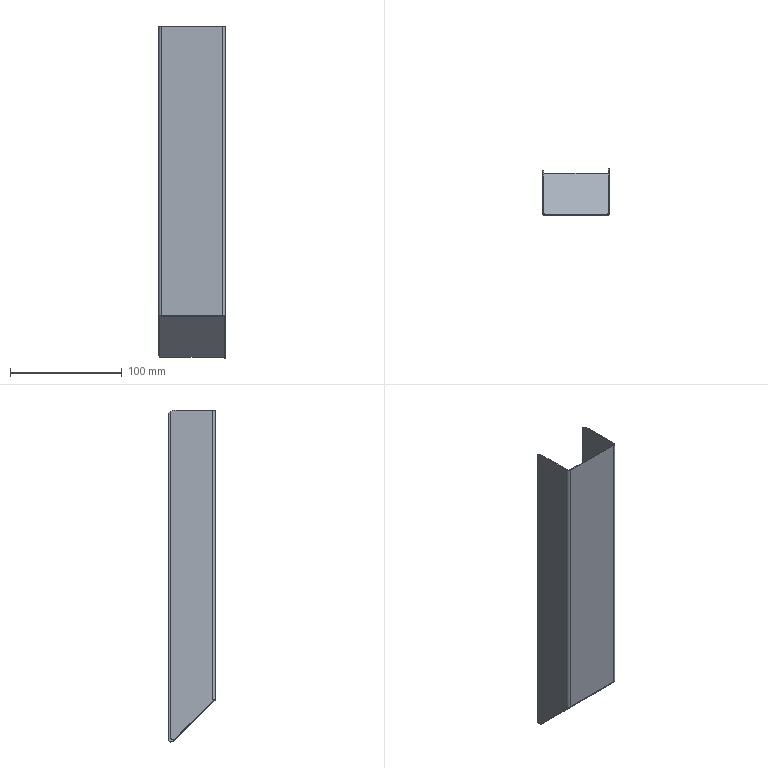Part | NX | 1 solid | 38 faces | box 60 x 42 x 297.657 mm | volume 40451 mm3 | plane 24 | cylinder 14 | commonest cylinder face diameters 4.5 x4 3.2 x2 4 x2 5.2 x2 20 x2 0.8 x1
STEP:
#1=CARTESIAN_POINT('',(1970.571,-113.09,-728.576));
#2=VERTEX_POINT('',#1);
#3=CARTESIAN_POINT('',(1970.571,-112.383,-727.869));
#4=VERTEX_POINT('',#3);
#5=CARTESIAN_POINT('',(1970.571,-112.383,-727.869));
#6=DIRECTION('',(0.,0.7071,0.7071));
#7=VECTOR('',#6,1000.);
#8=LINE('',#5,#7);
#9=EDGE_CURVE('',#2,#4,#8,.T.);
#10=ORIENTED_EDGE('',*,*,#9,.T.);
#11=CARTESIAN_POINT('',(1970.571,-75.621,-764.631));
#12=VERTEX_POINT('',#11);
#13=CARTESIAN_POINT('',(1970.571,-840.252,0.));
#14=DIRECTION('',(0.,-0.7071,0.7071));
#15=VECTOR('',#14,1000.);
#16=LINE('',#13,#15);
#17=EDGE_CURVE('',#12,#4,#16,.T.);
#18=ORIENTED_EDGE('',*,*,#17,.F.);
#19=CARTESIAN_POINT('',(1970.571,-76.328,-765.338));
#20=VERTEX_POINT('',#19);
#21=CARTESIAN_POINT('',(1970.571,0.,-689.01));
#22=DIRECTION('',(0.,-0.7071,-0.7071));
#23=VECTOR('',#22,1000.);
#24=LINE('',#21,#23);
#25=EDGE_CURVE('',#12,#20,#24,.T.);
#26=ORIENTED_EDGE('',*,*,#25,.T.);
#27=CARTESIAN_POINT('',(1970.571,-841.666,0.));
#28=DIRECTION('',(0.,-0.7071,0.7071));
#29=VECTOR('',#28,1000.);
#30=LINE('',#27,#29);
#31=EDGE_CURVE('',#20,#2,#30,.T.);
#32=ORIENTED_EDGE('',*,*,#31,.T.);
#33=EDGE_LOOP('',(#10,#18,#26,#32));
#34=FACE_BOUND('',#33,.T.);
#35=CARTESIAN_POINT('',(1970.571,-94.91,-745.342));
#36=DIRECTION('',(-1.,0.,0.));
#37=DIRECTION('',(0.,0.,1.));
#38=AXIS2_PLACEMENT_3D('',#35,#36,#37);
#39=PLANE('',#38);
#40=ADVANCED_FACE('',(#34),#39,.T.);
#41=CARTESIAN_POINT('',(2028.429,-112.383,-727.869));
#42=VERTEX_POINT('',#41);
#43=CARTESIAN_POINT('',(2028.429,-113.09,-728.576));
#44=VERTEX_POINT('',#43);
#45=CARTESIAN_POINT('',(2028.429,-112.383,-727.869));
#46=DIRECTION('',(0.,-0.7071,-0.7071));
#47=VECTOR('',#46,1000.);
#48=LINE('',#45,#47);
#49=EDGE_CURVE('',#42,#44,#48,.T.);
#50=ORIENTED_EDGE('',*,*,#49,.T.);
#51=CARTESIAN_POINT('',(2028.429,-76.328,-765.338));
#52=VERTEX_POINT('',#51);
#53=CARTESIAN_POINT('',(2028.429,-841.666,0.));
#54=DIRECTION('',(0.,0.7071,-0.7071));
#55=VECTOR('',#54,1000.);
#56=LINE('',#53,#55);
#57=EDGE_CURVE('',#44,#52,#56,.T.);
#58=ORIENTED_EDGE('',*,*,#57,.T.);
#59=CARTESIAN_POINT('',(2028.429,-75.621,-764.631));
#60=VERTEX_POINT('',#59);
#61=CARTESIAN_POINT('',(2028.429,0.,-689.01));
#62=DIRECTION('',(0.,0.7071,0.7071));
#63=VECTOR('',#62,1000.);
#64=LINE('',#61,#63);
#65=EDGE_CURVE('',#52,#60,#64,.T.);
#66=ORIENTED_EDGE('',*,*,#65,.T.);
#67=CARTESIAN_POINT('',(2028.429,-840.252,0.));
#68=DIRECTION('',(0.,0.7071,-0.7071));
#69=VECTOR('',#68,1000.);
#70=LINE('',#67,#69);
#71=EDGE_CURVE('',#42,#60,#70,.T.);
#72=ORIENTED_EDGE('',*,*,#71,.F.);
#73=EDGE_LOOP('',(#50,#58,#66,#72));
#74=FACE_BOUND('',#73,.T.);
#75=CARTESIAN_POINT('',(2028.429,-94.91,-745.342));
#76=DIRECTION('',(1.,0.,0.));
#77=DIRECTION('',(0.,1.,0.));
#78=AXIS2_PLACEMENT_3D('',#75,#76,#77);
#79=PLANE('',#78);
#80=ADVANCED_FACE('',(#74),#79,.T.);
#81=CARTESIAN_POINT('',(2026.9,-113.09,-728.576));
#82=VERTEX_POINT('',#81);
#83=CARTESIAN_POINT('',(2026.9,-113.5,-727.586));
#84=VERTEX_POINT('',#83);
#85=CARTESIAN_POINT('',(2026.9,-112.1,-727.586));
#86=DIRECTION('',(-1.,0.,0.));
#87=DIRECTION('',(0.,-0.7071,-0.7071));
#88=AXIS2_PLACEMENT_3D('',#85,#86,#87);
#89=CIRCLE('',#88,1.4);
#90=EDGE_CURVE('',#82,#84,#89,.T.);
#91=ORIENTED_EDGE('',*,*,#90,.F.);
#92=CARTESIAN_POINT('',(2026.9,-112.383,-727.869));
#93=VERTEX_POINT('',#92);
#94=CARTESIAN_POINT('',(2026.9,-113.09,-728.576));
#95=DIRECTION('',(0.,0.7071,0.7071));
#96=VECTOR('',#95,1000.);
#97=LINE('',#94,#96);
#98=EDGE_CURVE('',#82,#93,#97,.T.);
#99=ORIENTED_EDGE('',*,*,#98,.T.);
#100=CARTESIAN_POINT('',(2026.9,-112.5,-727.586));
#101=VERTEX_POINT('',#100);
#102=CARTESIAN_POINT('',(2026.9,-112.1,-727.586));
#103=DIRECTION('',(1.,0.,0.));
#104=DIRECTION('',(0.,-1.,0.));
#105=AXIS2_PLACEMENT_3D('',#102,#103,#104);
#106=CIRCLE('',#105,0.4);
#107=EDGE_CURVE('',#101,#93,#106,.T.);
#108=ORIENTED_EDGE('',*,*,#107,.F.);
#109=CARTESIAN_POINT('',(2026.9,-113.5,-727.586));
#110=DIRECTION('',(0.,1.,0.));
#111=VECTOR('',#110,1000.);
#112=LINE('',#109,#111);
#113=EDGE_CURVE('',#84,#101,#112,.T.);
#114=ORIENTED_EDGE('',*,*,#113,.F.);
#115=EDGE_LOOP('',(#91,#99,#108,#114));
#116=FACE_BOUND('',#115,.T.);
#117=CARTESIAN_POINT('',(2026.9,-112.1,-727.586));
#118=DIRECTION('',(-1.,0.,0.));
#119=DIRECTION('',(0.,0.,1.));
#120=AXIS2_PLACEMENT_3D('',#117,#118,#119);
#121=PLANE('',#120);
#122=ADVANCED_FACE('',(#116),#121,.F.);
#123=ORIENTED_EDGE('',*,*,#90,.T.);
#124=CARTESIAN_POINT('',(1972.1,-113.5,-727.586));
#125=VERTEX_POINT('',#124);
#126=CARTESIAN_POINT('',(1649.5,-113.5,-727.586));
#127=DIRECTION('',(1.,0.,0.));
#128=VECTOR('',#127,1000.);
#129=LINE('',#126,#128);
#130=EDGE_CURVE('',#125,#84,#129,.T.);
#131=ORIENTED_EDGE('',*,*,#130,.F.);
#132=CARTESIAN_POINT('',(1972.1,-113.09,-728.576));
#133=VERTEX_POINT('',#132);
#134=CARTESIAN_POINT('',(1972.1,-112.1,-727.586));
#135=DIRECTION('',(1.,0.,0.));
#136=DIRECTION('',(0.,-1.,0.));
#137=AXIS2_PLACEMENT_3D('',#134,#135,#136);
#138=CIRCLE('',#137,1.4);
#139=EDGE_CURVE('',#125,#133,#138,.T.);
#140=ORIENTED_EDGE('',*,*,#139,.T.);
#141=CARTESIAN_POINT('',(1649.5,-113.09,-728.576));
#142=DIRECTION('',(1.,0.,0.));
#143=VECTOR('',#142,1000.);
#144=LINE('',#141,#143);
#145=EDGE_CURVE('',#133,#82,#144,.T.);
#146=ORIENTED_EDGE('',*,*,#145,.T.);
#147=EDGE_LOOP('',(#123,#131,#140,#146));
#148=FACE_BOUND('',#147,.T.);
#149=CARTESIAN_POINT('',(1972.1,-112.1,-727.586));
#150=DIRECTION('',(-1.,0.,0.));
#151=DIRECTION('',(0.,0.,-1.));
#152=AXIS2_PLACEMENT_3D('',#149,#150,#151);
#153=CYLINDRICAL_SURFACE('',#152,1.4);
#154=ADVANCED_FACE('',(#148),#153,.T.);
#155=CARTESIAN_POINT('',(1649.5,-113.09,-728.576));
#156=DIRECTION('',(-1.,0.,0.));
#157=VECTOR('',#156,1000.);
#158=LINE('',#155,#157);
#159=EDGE_CURVE('',#44,#82,#158,.T.);
#160=ORIENTED_EDGE('',*,*,#159,.T.);
#161=ORIENTED_EDGE('',*,*,#145,.F.);
#162=CARTESIAN_POINT('',(1649.5,-113.09,-728.576));
#163=DIRECTION('',(-1.,0.,0.));
#164=VECTOR('',#163,1000.);
#165=LINE('',#162,#164);
#166=EDGE_CURVE('',#133,#2,#165,.T.);
#167=ORIENTED_EDGE('',*,*,#166,.T.);
#168=ORIENTED_EDGE('',*,*,#31,.F.);
#169=CARTESIAN_POINT('',(0.,-76.328,-765.338));
#170=DIRECTION('',(-1.,0.,0.));
#171=VECTOR('',#170,1000.);
#172=LINE('',#169,#171);
#173=EDGE_CURVE('',#52,#20,#172,.T.);
#174=ORIENTED_EDGE('',*,*,#173,.F.);
#175=ORIENTED_EDGE('',*,*,#57,.F.);
#176=EDGE_LOOP('',(#160,#161,#167,#168,#174,#175));
#177=FACE_BOUND('',#176,.T.);
#178=CARTESIAN_POINT('',(1649.5,-325.159,-516.507));
#179=DIRECTION('',(0.,0.7071,0.7071));
#180=DIRECTION('',(1.,0.,0.));
#181=AXIS2_PLACEMENT_3D('',#178,#179,#180);
#182=PLANE('',#181);
#183=ADVANCED_FACE('',(#177),#182,.F.);
#184=ORIENTED_EDGE('',*,*,#166,.F.);
#185=CARTESIAN_POINT('',(1972.1,-112.383,-727.869));
#186=VERTEX_POINT('',#185);
#187=CARTESIAN_POINT('',(1972.1,-113.09,-728.576));
#188=DIRECTION('',(0.,0.7071,0.7071));
#189=VECTOR('',#188,1000.);
#190=LINE('',#187,#189);
#191=EDGE_CURVE('',#133,#186,#190,.T.);
#192=ORIENTED_EDGE('',*,*,#191,.T.);
#193=CARTESIAN_POINT('',(1649.5,-112.383,-727.869));
#194=DIRECTION('',(1.,0.,0.));
#195=VECTOR('',#194,1000.);
#196=LINE('',#193,#195);
#197=EDGE_CURVE('',#4,#186,#196,.T.);
#198=ORIENTED_EDGE('',*,*,#197,.F.);
#199=ORIENTED_EDGE('',*,*,#9,.F.);
#200=EDGE_LOOP('',(#184,#192,#198,#199));
#201=FACE_BOUND('',#200,.T.);
#202=CARTESIAN_POINT('',(1972.1,-113.09,-728.576));
#203=DIRECTION('',(0.,-0.7071,0.7071));
#204=DIRECTION('',(-1.,0.,0.));
#205=AXIS2_PLACEMENT_3D('',#202,#203,#204);
#206=PLANE('',#205);
#207=ADVANCED_FACE('',(#201),#206,.T.);
#208=ORIENTED_EDGE('',*,*,#139,.F.);
#209=CARTESIAN_POINT('',(1972.1,-112.5,-727.586));
#210=VERTEX_POINT('',#209);
#211=CARTESIAN_POINT('',(1972.1,-113.5,-727.586));
#212=DIRECTION('',(0.,1.,0.));
#213=VECTOR('',#212,1000.);
#214=LINE('',#211,#213);
#215=EDGE_CURVE('',#125,#210,#214,.T.);
#216=ORIENTED_EDGE('',*,*,#215,.T.);
#217=CARTESIAN_POINT('',(1972.1,-112.1,-727.586));
#218=DIRECTION('',(-1.,0.,0.));
#219=DIRECTION('',(0.,-0.7071,-0.7071));
#220=AXIS2_PLACEMENT_3D('',#217,#218,#219);
#221=CIRCLE('',#220,0.4);
#222=EDGE_CURVE('',#186,#210,#221,.T.);
#223=ORIENTED_EDGE('',*,*,#222,.F.);
#224=ORIENTED_EDGE('',*,*,#191,.F.);
#225=EDGE_LOOP('',(#208,#216,#223,#224));
#226=FACE_BOUND('',#225,.T.);
#227=CARTESIAN_POINT('',(1972.1,-112.1,-727.586));
#228=DIRECTION('',(1.,0.,0.));
#229=DIRECTION('',(0.,1.,0.));
#230=AXIS2_PLACEMENT_3D('',#227,#228,#229);
#231=PLANE('',#230);
#232=ADVANCED_FACE('',(#226),#231,.F.);
#233=CARTESIAN_POINT('',(1969.5,-110.9,-727.586));
#234=VERTEX_POINT('',#233);
#235=CARTESIAN_POINT('',(1972.1,-110.9,-727.586));
#236=DIRECTION('',(0.,0.,1.));
#237=DIRECTION('',(-1.,0.,0.));
#238=AXIS2_PLACEMENT_3D('',#235,#236,#237);
#239=CIRCLE('',#238,2.6);
#240=EDGE_CURVE('',#234,#125,#239,.T.);
#241=ORIENTED_EDGE('',*,*,#240,.F.);
#242=CARTESIAN_POINT('',(1970.5,-110.9,-727.586));
#243=VERTEX_POINT('',#242);
#244=CARTESIAN_POINT('',(1969.5,-110.9,-727.586));
#245=DIRECTION('',(1.,0.,0.));
#246=VECTOR('',#245,1000.);
#247=LINE('',#244,#246);
#248=EDGE_CURVE('',#234,#243,#247,.T.);
#249=ORIENTED_EDGE('',*,*,#248,.T.);
#250=CARTESIAN_POINT('',(1972.1,-110.9,-727.586));
#251=DIRECTION('',(0.,0.,-1.));
#252=DIRECTION('',(0.,-1.,0.));
#253=AXIS2_PLACEMENT_3D('',#250,#251,#252);
#254=CIRCLE('',#253,1.6);
#255=EDGE_CURVE('',#210,#243,#254,.T.);
#256=ORIENTED_EDGE('',*,*,#255,.F.);
#257=ORIENTED_EDGE('',*,*,#215,.F.);
#258=EDGE_LOOP('',(#241,#249,#256,#257));
#259=FACE_BOUND('',#258,.T.);
#260=CARTESIAN_POINT('',(1972.1,-110.9,-727.586));
#261=DIRECTION('',(0.,0.,1.));
#262=DIRECTION('',(1.,0.,0.));
#263=AXIS2_PLACEMENT_3D('',#260,#261,#262);
#264=PLANE('',#263);
#265=ADVANCED_FACE('',(#259),#264,.F.);
#266=CARTESIAN_POINT('',(1972.1,-113.5,-468.166));
#267=VERTEX_POINT('',#266);
#268=CARTESIAN_POINT('',(1972.1,-113.5,-428.166));
#269=DIRECTION('',(0.,0.,-1.));
#270=VECTOR('',#269,1000.);
#271=LINE('',#268,#270);
#272=EDGE_CURVE('',#267,#125,#271,.T.);
#273=ORIENTED_EDGE('',*,*,#272,.F.);
#274=CARTESIAN_POINT('',(1969.5,-110.9,-468.166));
#275=VERTEX_POINT('',#274);
#276=CARTESIAN_POINT('',(1972.1,-110.9,-468.166));
#277=DIRECTION('',(0.,0.,1.));
#278=DIRECTION('',(-1.,0.,0.));
#279=AXIS2_PLACEMENT_3D('',#276,#277,#278);
#280=CIRCLE('',#279,2.6);
#281=EDGE_CURVE('',#275,#267,#280,.T.);
#282=ORIENTED_EDGE('',*,*,#281,.F.);
#283=CARTESIAN_POINT('',(1969.5,-110.9,-578.166));
#284=DIRECTION('',(0.,0.,1.));
#285=VECTOR('',#284,1000.);
#286=LINE('',#283,#285);
#287=EDGE_CURVE('',#234,#275,#286,.T.);
#288=ORIENTED_EDGE('',*,*,#287,.F.);
#289=ORIENTED_EDGE('',*,*,#240,.T.);
#290=EDGE_LOOP('',(#273,#282,#288,#289));
#291=FACE_BOUND('',#290,.T.);
#292=CARTESIAN_POINT('',(1972.1,-110.9,-578.166));
#293=DIRECTION('',(0.,0.,1.));
#294=DIRECTION('',(-1.,0.,0.));
#295=AXIS2_PLACEMENT_3D('',#292,#293,#294);
#296=CYLINDRICAL_SURFACE('',#295,2.6);
#297=ADVANCED_FACE('',(#291),#296,.T.);
#298=ORIENTED_EDGE('',*,*,#287,.T.);
#299=CARTESIAN_POINT('',(1969.5,-78.5,-468.166));
#300=VERTEX_POINT('',#299);
#301=CARTESIAN_POINT('',(1969.5,-112.5,-468.166));
#302=DIRECTION('',(0.,-1.,0.));
#303=VECTOR('',#302,1000.);
#304=LINE('',#301,#303);
#305=EDGE_CURVE('',#300,#275,#304,.T.);
#306=ORIENTED_EDGE('',*,*,#305,.F.);
#307=CARTESIAN_POINT('',(1969.5,-73.5,-469.506));
#308=VERTEX_POINT('',#307);
#309=CARTESIAN_POINT('',(1969.5,-78.5,-478.166));
#310=DIRECTION('',(1.,0.,0.));
#311=DIRECTION('',(0.,0.,1.));
#312=AXIS2_PLACEMENT_3D('',#309,#310,#311);
#313=CIRCLE('',#312,10.);
#314=EDGE_CURVE('',#308,#300,#313,.T.);
#315=ORIENTED_EDGE('',*,*,#314,.F.);
#316=CARTESIAN_POINT('',(1969.5,-73.5,-761.824));
#317=VERTEX_POINT('',#316);
#318=CARTESIAN_POINT('',(1969.5,-73.5,0.));
#319=DIRECTION('',(0.,0.,1.));
#320=VECTOR('',#319,1000.);
#321=LINE('',#318,#320);
#322=EDGE_CURVE('',#317,#308,#321,.T.);
#323=ORIENTED_EDGE('',*,*,#322,.F.);
#324=CARTESIAN_POINT('',(1969.5,-76.914,-763.238));
#325=VERTEX_POINT('',#324);
#326=CARTESIAN_POINT('',(1969.5,-75.5,-761.824));
#327=DIRECTION('',(1.,0.,0.));
#328=DIRECTION('',(0.,-1.,0.));
#329=AXIS2_PLACEMENT_3D('',#326,#327,#328);
#330=CIRCLE('',#329,2.);
#331=EDGE_CURVE('',#325,#317,#330,.T.);
#332=ORIENTED_EDGE('',*,*,#331,.F.);
#333=CARTESIAN_POINT('',(1969.5,-110.9,-729.252));
#334=VERTEX_POINT('',#333);
#335=CARTESIAN_POINT('',(1969.5,0.,-840.152));
#336=DIRECTION('',(0.,0.7071,-0.7071));
#337=VECTOR('',#336,1000.);
#338=LINE('',#335,#337);
#339=EDGE_CURVE('',#334,#325,#338,.T.);
#340=ORIENTED_EDGE('',*,*,#339,.F.);
#341=CARTESIAN_POINT('',(1969.5,-110.9,-428.166));
#342=DIRECTION('',(0.,0.,-1.));
#343=VECTOR('',#342,1000.);
#344=LINE('',#341,#343);
#345=EDGE_CURVE('',#234,#334,#344,.T.);
#346=ORIENTED_EDGE('',*,*,#345,.F.);
#347=EDGE_LOOP('',(#298,#306,#315,#323,#332,#340,#346));
#348=FACE_BOUND('',#347,.T.);
#349=CARTESIAN_POINT('',(1969.5,208.6,-428.166));
#350=DIRECTION('',(1.,0.,0.));
#351=DIRECTION('',(0.,1.,0.));
#352=AXIS2_PLACEMENT_3D('',#349,#350,#351);
#353=PLANE('',#352);
#354=ADVANCED_FACE('',(#348),#353,.F.);
#355=ORIENTED_EDGE('',*,*,#173,.T.);
#356=ORIENTED_EDGE('',*,*,#25,.F.);
#357=CARTESIAN_POINT('',(0.,-75.621,-764.631));
#358=DIRECTION('',(-1.,0.,0.));
#359=VECTOR('',#358,1000.);
#360=LINE('',#357,#359);
#361=EDGE_CURVE('',#60,#12,#360,.T.);
#362=ORIENTED_EDGE('',*,*,#361,.F.);
#363=ORIENTED_EDGE('',*,*,#65,.F.);
#364=EDGE_LOOP('',(#355,#356,#362,#363));
#365=FACE_BOUND('',#364,.T.);
#366=CARTESIAN_POINT('',(1969.5,-76.328,-765.338));
#367=DIRECTION('',(0.,0.7071,-0.7071));
#368=DIRECTION('',(-1.,0.,0.));
#369=AXIS2_PLACEMENT_3D('',#366,#367,#368);
#370=PLANE('',#369);
#371=ADVANCED_FACE('',(#365),#370,.T.);
#372=CARTESIAN_POINT('',(1970.5,-76.914,-763.238));
#373=VERTEX_POINT('',#372);
#374=CARTESIAN_POINT('',(0.,-76.914,-763.238));
#375=DIRECTION('',(1.,0.,0.));
#376=VECTOR('',#375,1000.);
#377=LINE('',#374,#376);
#378=EDGE_CURVE('',#325,#373,#377,.T.);
#379=ORIENTED_EDGE('',*,*,#378,.T.);
#380=CARTESIAN_POINT('',(1970.5,-110.9,-729.252));
#381=VERTEX_POINT('',#380);
#382=CARTESIAN_POINT('',(1970.5,0.,-840.152));
#383=DIRECTION('',(0.,0.7071,-0.7071));
#384=VECTOR('',#383,1000.);
#385=LINE('',#382,#384);
#386=EDGE_CURVE('',#381,#373,#385,.T.);
#387=ORIENTED_EDGE('',*,*,#386,.F.);
#388=CARTESIAN_POINT('',(1969.5,-110.9,-729.252));
#389=DIRECTION('',(1.,0.,0.));
#390=VECTOR('',#389,1000.);
#391=LINE('',#388,#390);
#392=EDGE_CURVE('',#334,#381,#391,.T.);
#393=ORIENTED_EDGE('',*,*,#392,.F.);
#394=ORIENTED_EDGE('',*,*,#339,.T.);
#395=EDGE_LOOP('',(#379,#387,#393,#394));
#396=FACE_BOUND('',#395,.T.);
#397=CARTESIAN_POINT('',(1969.5,-68.5,-771.652));
#398=DIRECTION('',(0.,-0.7071,-0.7071));
#399=DIRECTION('',(0.,-0.7071,0.7071));
#400=AXIS2_PLACEMENT_3D('',#397,#398,#399);
#401=PLANE('',#400);
#402=ADVANCED_FACE('',(#396),#401,.T.);
#403=CARTESIAN_POINT('',(1970.5,-73.5,-469.506));
#404=VERTEX_POINT('',#403);
#405=CARTESIAN_POINT('',(1649.5,-73.5,-469.506));
#406=DIRECTION('',(1.,0.,0.));
#407=VECTOR('',#406,1000.);
#408=LINE('',#405,#407);
#409=EDGE_CURVE('',#308,#404,#408,.T.);
#410=ORIENTED_EDGE('',*,*,#409,.T.);
#411=CARTESIAN_POINT('',(1970.5,-73.5,-761.824));
#412=VERTEX_POINT('',#411);
#413=CARTESIAN_POINT('',(1970.5,-73.5,0.));
#414=DIRECTION('',(0.,0.,1.));
#415=VECTOR('',#414,1000.);
#416=LINE('',#413,#415);
#417=EDGE_CURVE('',#412,#404,#416,.T.);
#418=ORIENTED_EDGE('',*,*,#417,.F.);
#419=CARTESIAN_POINT('',(0.,-73.5,-761.824));
#420=DIRECTION('',(1.,0.,0.));
#421=VECTOR('',#420,1000.);
#422=LINE('',#419,#421);
#423=EDGE_CURVE('',#317,#412,#422,.T.);
#424=ORIENTED_EDGE('',*,*,#423,.F.);
#425=ORIENTED_EDGE('',*,*,#322,.T.);
#426=EDGE_LOOP('',(#410,#418,#424,#425));
#427=FACE_BOUND('',#426,.T.);
#428=CARTESIAN_POINT('',(1969.5,-73.5,-578.166));
#429=DIRECTION('',(0.,1.,0.));
#430=DIRECTION('',(1.,0.,0.));
#431=AXIS2_PLACEMENT_3D('',#428,#429,#430);
#432=PLANE('',#431);
#433=ADVANCED_FACE('',(#427),#432,.T.);
#434=ORIENTED_EDGE('',*,*,#345,.T.);
#435=ORIENTED_EDGE('',*,*,#392,.T.);
#436=CARTESIAN_POINT('',(1970.5,-110.9,-428.166));
#437=DIRECTION('',(0.,0.,-1.));
#438=VECTOR('',#437,1000.);
#439=LINE('',#436,#438);
#440=EDGE_CURVE('',#243,#381,#439,.T.);
#441=ORIENTED_EDGE('',*,*,#440,.F.);
#442=ORIENTED_EDGE('',*,*,#248,.F.);
#443=EDGE_LOOP('',(#434,#435,#441,#442));
#444=FACE_BOUND('',#443,.T.);
#445=CARTESIAN_POINT('',(1969.5,-110.9,-728.078));
#446=DIRECTION('',(0.,-1.,0.));
#447=DIRECTION('',(-1.,0.,0.));
#448=AXIS2_PLACEMENT_3D('',#445,#446,#447);
#449=PLANE('',#448);
#450=ADVANCED_FACE('',(#444),#449,.T.);
#451=ORIENTED_EDGE('',*,*,#409,.F.);
#452=ORIENTED_EDGE('',*,*,#314,.T.);
#453=CARTESIAN_POINT('',(1970.5,-78.5,-468.166));
#454=VERTEX_POINT('',#453);
#455=CARTESIAN_POINT('',(1649.5,-78.5,-468.166));
#456=DIRECTION('',(1.,0.,0.));
#457=VECTOR('',#456,1000.);
#458=LINE('',#455,#457);
#459=EDGE_CURVE('',#300,#454,#458,.T.);
#460=ORIENTED_EDGE('',*,*,#459,.T.);
#461=CARTESIAN_POINT('',(1970.5,-78.5,-478.166));
#462=DIRECTION('',(1.,0.,0.));
#463=DIRECTION('',(0.,0.,1.));
#464=AXIS2_PLACEMENT_3D('',#461,#462,#463);
#465=CIRCLE('',#464,10.);
#466=EDGE_CURVE('',#404,#454,#465,.T.);
#467=ORIENTED_EDGE('',*,*,#466,.F.);
#468=EDGE_LOOP('',(#451,#452,#460,#467));
#469=FACE_BOUND('',#468,.T.);
#470=CARTESIAN_POINT('',(1649.5,-78.5,-478.166));
#471=DIRECTION('',(1.,0.,0.));
#472=DIRECTION('',(0.,0.,1.));
#473=AXIS2_PLACEMENT_3D('',#470,#471,#472);
#474=CYLINDRICAL_SURFACE('',#473,10.);
#475=ADVANCED_FACE('',(#469),#474,.T.);
#476=ORIENTED_EDGE('',*,*,#159,.F.);
#477=ORIENTED_EDGE('',*,*,#49,.F.);
#478=CARTESIAN_POINT('',(1649.5,-112.383,-727.869));
#479=DIRECTION('',(1.,0.,0.));
#480=VECTOR('',#479,1000.);
#481=LINE('',#478,#480);
#482=EDGE_CURVE('',#93,#42,#481,.T.);
#483=ORIENTED_EDGE('',*,*,#482,.F.);
#484=ORIENTED_EDGE('',*,*,#98,.F.);
#485=EDGE_LOOP('',(#476,#477,#483,#484));
#486=FACE_BOUND('',#485,.T.);
#487=CARTESIAN_POINT('',(2030.,-113.09,-728.576));
#488=DIRECTION('',(0.,-0.7071,0.7071));
#489=DIRECTION('',(-1.,0.,0.));
#490=AXIS2_PLACEMENT_3D('',#487,#488,#489);
#491=PLANE('',#490);
#492=ADVANCED_FACE('',(#486),#491,.T.);
#493=CARTESIAN_POINT('',(2029.5,-110.9,-727.586));
#494=VERTEX_POINT('',#493);
#495=CARTESIAN_POINT('',(2026.9,-110.9,-727.586));
#496=DIRECTION('',(0.,0.,1.));
#497=DIRECTION('',(0.,-1.,0.));
#498=AXIS2_PLACEMENT_3D('',#495,#496,#497);
#499=CIRCLE('',#498,2.6);
#500=EDGE_CURVE('',#84,#494,#499,.T.);
#501=ORIENTED_EDGE('',*,*,#500,.F.);
#502=ORIENTED_EDGE('',*,*,#113,.T.);
#503=CARTESIAN_POINT('',(2028.5,-110.9,-727.586));
#504=VERTEX_POINT('',#503);
#505=CARTESIAN_POINT('',(2026.9,-110.9,-727.586));
#506=DIRECTION('',(0.,0.,-1.));
#507=DIRECTION('',(1.,0.,0.));
#508=AXIS2_PLACEMENT_3D('',#505,#506,#507);
#509=CIRCLE('',#508,1.6);
#510=EDGE_CURVE('',#504,#101,#509,.T.);
#511=ORIENTED_EDGE('',*,*,#510,.F.);
#512=CARTESIAN_POINT('',(2029.5,-110.9,-727.586));
#513=DIRECTION('',(-1.,0.,0.));
#514=VECTOR('',#513,1000.);
#515=LINE('',#512,#514);
#516=EDGE_CURVE('',#494,#504,#515,.T.);
#517=ORIENTED_EDGE('',*,*,#516,.F.);
#518=EDGE_LOOP('',(#501,#502,#511,#517));
#519=FACE_BOUND('',#518,.T.);
#520=CARTESIAN_POINT('',(2026.9,-110.9,-727.586));
#521=DIRECTION('',(0.,0.,1.));
#522=DIRECTION('',(1.,0.,0.));
#523=AXIS2_PLACEMENT_3D('',#520,#521,#522);
#524=PLANE('',#523);
#525=ADVANCED_FACE('',(#519),#524,.F.);
#526=CARTESIAN_POINT('',(2028.5,-74.914,-765.238));
#527=VERTEX_POINT('',#526);
#528=CARTESIAN_POINT('',(2029.5,-74.914,-765.238));
#529=VERTEX_POINT('',#528);
#530=CARTESIAN_POINT('',(0.,-74.914,-765.238));
#531=DIRECTION('',(1.,0.,0.));
#532=VECTOR('',#531,1000.);
#533=LINE('',#530,#532);
#534=EDGE_CURVE('',#527,#529,#533,.T.);
#535=ORIENTED_EDGE('',*,*,#534,.T.);
#536=CARTESIAN_POINT('',(2029.5,-110.9,-729.252));
#537=VERTEX_POINT('',#536);
#538=CARTESIAN_POINT('',(2029.5,-840.152,0.));
#539=DIRECTION('',(0.,-0.7071,0.7071));
#540=VECTOR('',#539,1000.);
#541=LINE('',#538,#540);
#542=EDGE_CURVE('',#529,#537,#541,.T.);
#543=ORIENTED_EDGE('',*,*,#542,.T.);
#544=CARTESIAN_POINT('',(2028.5,-110.9,-729.252));
#545=VERTEX_POINT('',#544);
#546=CARTESIAN_POINT('',(2029.5,-110.9,-729.252));
#547=DIRECTION('',(1.,0.,0.));
#548=VECTOR('',#547,1000.);
#549=LINE('',#546,#548);
#550=EDGE_CURVE('',#545,#537,#549,.T.);
#551=ORIENTED_EDGE('',*,*,#550,.F.);
#552=CARTESIAN_POINT('',(2028.5,-840.152,0.));
#553=DIRECTION('',(0.,-0.7071,0.7071));
#554=VECTOR('',#553,1000.);
#555=LINE('',#552,#554);
#556=EDGE_CURVE('',#527,#545,#555,.T.);
#557=ORIENTED_EDGE('',*,*,#556,.F.);
#558=EDGE_LOOP('',(#535,#543,#551,#557));
#559=FACE_BOUND('',#558,.T.);
#560=CARTESIAN_POINT('',(2029.5,-111.4,-728.752));
#561=DIRECTION('',(0.,-0.7071,-0.7071));
#562=DIRECTION('',(0.,0.7071,-0.7071));
#563=AXIS2_PLACEMENT_3D('',#560,#561,#562);
#564=PLANE('',#563);
#565=ADVANCED_FACE('',(#559),#564,.T.);
#566=CARTESIAN_POINT('',(2029.5,-71.5,-763.824));
#567=VERTEX_POINT('',#566);
#568=CARTESIAN_POINT('',(2029.5,-71.5,-471.025));
#569=VERTEX_POINT('',#568);
#570=CARTESIAN_POINT('',(2029.5,-71.5,0.));
#571=DIRECTION('',(0.,0.,1.));
#572=VECTOR('',#571,1000.);
#573=LINE('',#570,#572);
#574=EDGE_CURVE('',#567,#569,#573,.T.);
#575=ORIENTED_EDGE('',*,*,#574,.F.);
#576=CARTESIAN_POINT('',(2028.5,-71.5,-763.824));
#577=VERTEX_POINT('',#576);
#578=CARTESIAN_POINT('',(0.,-71.5,-763.824));
#579=DIRECTION('',(1.,0.,0.));
#580=VECTOR('',#579,1000.);
#581=LINE('',#578,#580);
#582=EDGE_CURVE('',#577,#567,#581,.T.);
#583=ORIENTED_EDGE('',*,*,#582,.F.);
#584=CARTESIAN_POINT('',(2028.5,-71.5,-471.025));
#585=VERTEX_POINT('',#584);
#586=CARTESIAN_POINT('',(2028.5,-71.5,0.));
#587=DIRECTION('',(0.,0.,-1.));
#588=VECTOR('',#587,1000.);
#589=LINE('',#586,#588);
#590=EDGE_CURVE('',#585,#577,#589,.T.);
#591=ORIENTED_EDGE('',*,*,#590,.F.);
#592=CARTESIAN_POINT('',(1649.5,-71.5,-471.025));
#593=DIRECTION('',(1.,0.,0.));
#594=VECTOR('',#593,1000.);
#595=LINE('',#592,#594);
#596=EDGE_CURVE('',#585,#569,#595,.T.);
#597=ORIENTED_EDGE('',*,*,#596,.T.);
#598=EDGE_LOOP('',(#575,#583,#591,#597));
#599=FACE_BOUND('',#598,.T.);
#600=CARTESIAN_POINT('',(2029.5,-71.5,-771.652));
#601=DIRECTION('',(0.,1.,0.));
#602=DIRECTION('',(1.,0.,0.));
#603=AXIS2_PLACEMENT_3D('',#600,#601,#602);
#604=PLANE('',#603);
#605=ADVANCED_FACE('',(#599),#604,.T.);
#606=ORIENTED_EDGE('',*,*,#500,.T.);
#607=CARTESIAN_POINT('',(2029.5,-110.9,-468.166));
#608=VERTEX_POINT('',#607);
#609=CARTESIAN_POINT('',(2029.5,-110.9,-727.586));
#610=DIRECTION('',(0.,0.,-1.));
#611=VECTOR('',#610,1000.);
#612=LINE('',#609,#611);
#613=EDGE_CURVE('',#608,#494,#612,.T.);
#614=ORIENTED_EDGE('',*,*,#613,.F.);
#615=CARTESIAN_POINT('',(2026.9,-113.5,-468.166));
#616=VERTEX_POINT('',#615);
#617=CARTESIAN_POINT('',(2026.9,-110.9,-468.166));
#618=DIRECTION('',(0.,0.,-1.));
#619=DIRECTION('',(1.,0.,0.));
#620=AXIS2_PLACEMENT_3D('',#617,#618,#619);
#621=CIRCLE('',#620,2.6);
#622=EDGE_CURVE('',#608,#616,#621,.T.);
#623=ORIENTED_EDGE('',*,*,#622,.T.);
#624=CARTESIAN_POINT('',(2026.9,-113.5,-428.166));
#625=DIRECTION('',(0.,0.,-1.));
#626=VECTOR('',#625,1000.);
#627=LINE('',#624,#626);
#628=EDGE_CURVE('',#616,#84,#627,.T.);
#629=ORIENTED_EDGE('',*,*,#628,.T.);
#630=EDGE_LOOP('',(#606,#614,#623,#629));
#631=FACE_BOUND('',#630,.T.);
#632=CARTESIAN_POINT('',(2026.9,-110.9,-727.586));
#633=DIRECTION('',(0.,0.,-1.));
#634=DIRECTION('',(1.,0.,0.));
#635=AXIS2_PLACEMENT_3D('',#632,#633,#634);
#636=CYLINDRICAL_SURFACE('',#635,2.6);
#637=ADVANCED_FACE('',(#631),#636,.T.);
#638=CARTESIAN_POINT('',(2028.5,-78.5,-468.166));
#639=VERTEX_POINT('',#638);
#640=CARTESIAN_POINT('',(2029.5,-78.5,-468.166));
#641=VERTEX_POINT('',#640);
#642=CARTESIAN_POINT('',(1649.5,-78.5,-468.166));
#643=DIRECTION('',(1.,0.,0.));
#644=VECTOR('',#643,1000.);
#645=LINE('',#642,#644);
#646=EDGE_CURVE('',#639,#641,#645,.T.);
#647=ORIENTED_EDGE('',*,*,#646,.F.);
#648=CARTESIAN_POINT('',(2028.5,-110.9,-468.166));
#649=VERTEX_POINT('',#648);
#650=CARTESIAN_POINT('',(2028.5,-112.5,-468.166));
#651=DIRECTION('',(0.,1.,0.));
#652=VECTOR('',#651,1000.);
#653=LINE('',#650,#652);
#654=EDGE_CURVE('',#649,#639,#653,.T.);
#655=ORIENTED_EDGE('',*,*,#654,.F.);
#656=CARTESIAN_POINT('',(2026.9,-112.5,-468.166));
#657=VERTEX_POINT('',#656);
#658=CARTESIAN_POINT('',(2026.9,-110.9,-468.166));
#659=DIRECTION('',(0.,0.,-1.));
#660=DIRECTION('',(1.,0.,0.));
#661=AXIS2_PLACEMENT_3D('',#658,#659,#660);
#662=CIRCLE('',#661,1.6);
#663=EDGE_CURVE('',#649,#657,#662,.T.);
#664=ORIENTED_EDGE('',*,*,#663,.T.);
#665=CARTESIAN_POINT('',(1972.1,-112.5,-468.166));
#666=VERTEX_POINT('',#665);
#667=CARTESIAN_POINT('',(1649.5,-112.5,-468.166));
#668=DIRECTION('',(1.,0.,0.));
#669=VECTOR('',#668,1000.);
#670=LINE('',#667,#669);
#671=EDGE_CURVE('',#666,#657,#670,.T.);
#672=ORIENTED_EDGE('',*,*,#671,.F.);
#673=CARTESIAN_POINT('',(1970.5,-110.9,-468.166));
#674=VERTEX_POINT('',#673);
#675=CARTESIAN_POINT('',(1972.1,-110.9,-468.166));
#676=DIRECTION('',(0.,0.,1.));
#677=DIRECTION('',(-1.,0.,0.));
#678=AXIS2_PLACEMENT_3D('',#675,#676,#677);
#679=CIRCLE('',#678,1.6);
#680=EDGE_CURVE('',#674,#666,#679,.T.);
#681=ORIENTED_EDGE('',*,*,#680,.F.);
#682=CARTESIAN_POINT('',(1970.5,-112.5,-468.166));
#683=DIRECTION('',(0.,-1.,0.));
#684=VECTOR('',#683,1000.);
#685=LINE('',#682,#684);
#686=EDGE_CURVE('',#454,#674,#685,.T.);
#687=ORIENTED_EDGE('',*,*,#686,.F.);
#688=ORIENTED_EDGE('',*,*,#459,.F.);
#689=ORIENTED_EDGE('',*,*,#305,.T.);
#690=ORIENTED_EDGE('',*,*,#281,.T.);
#691=CARTESIAN_POINT('',(1649.5,-113.5,-468.166));
#692=DIRECTION('',(-1.,0.,0.));
#693=VECTOR('',#692,1000.);
#694=LINE('',#691,#693);
#695=EDGE_CURVE('',#616,#267,#694,.T.);
#696=ORIENTED_EDGE('',*,*,#695,.F.);
#697=ORIENTED_EDGE('',*,*,#622,.F.);
#698=CARTESIAN_POINT('',(2029.5,-112.5,-468.166));
#699=DIRECTION('',(0.,-1.,0.));
#700=VECTOR('',#699,1000.);
#701=LINE('',#698,#700);
#702=EDGE_CURVE('',#641,#608,#701,.T.);
#703=ORIENTED_EDGE('',*,*,#702,.F.);
#704=EDGE_LOOP('',(#647,#655,#664,#672,#681,#687,#688,#689,#690,#696,#697,#703));
#705=FACE_BOUND('',#704,.T.);
#706=CARTESIAN_POINT('',(2029.5,-68.5,-468.166));
#707=DIRECTION('',(0.,0.,1.));
#708=DIRECTION('',(0.,-1.,0.));
#709=AXIS2_PLACEMENT_3D('',#706,#707,#708);
#710=PLANE('',#709);
#711=ADVANCED_FACE('',(#705),#710,.T.);
#712=CARTESIAN_POINT('',(2029.5,-110.9,-428.166));
#713=DIRECTION('',(0.,0.,-1.));
#714=VECTOR('',#713,1000.);
#715=LINE('',#712,#714);
#716=EDGE_CURVE('',#494,#537,#715,.T.);
#717=ORIENTED_EDGE('',*,*,#716,.F.);
#718=ORIENTED_EDGE('',*,*,#516,.T.);
#719=CARTESIAN_POINT('',(2028.5,-110.9,-428.166));
#720=DIRECTION('',(0.,0.,1.));
#721=VECTOR('',#720,1000.);
#722=LINE('',#719,#721);
#723=EDGE_CURVE('',#545,#504,#722,.T.);
#724=ORIENTED_EDGE('',*,*,#723,.F.);
#725=ORIENTED_EDGE('',*,*,#550,.T.);
#726=EDGE_LOOP('',(#717,#718,#724,#725));
#727=FACE_BOUND('',#726,.T.);
#728=CARTESIAN_POINT('',(2029.5,-110.9,-727.586));
#729=DIRECTION('',(0.,-1.,0.));
#730=DIRECTION('',(-1.,0.,0.));
#731=AXIS2_PLACEMENT_3D('',#728,#729,#730);
#732=PLANE('',#731);
#733=ADVANCED_FACE('',(#727),#732,.T.);
#734=ORIENTED_EDGE('',*,*,#628,.F.);
#735=ORIENTED_EDGE('',*,*,#695,.T.);
#736=ORIENTED_EDGE('',*,*,#272,.T.);
#737=ORIENTED_EDGE('',*,*,#130,.T.);
#738=EDGE_LOOP('',(#734,#735,#736,#737));
#739=FACE_BOUND('',#738,.T.);
#740=CARTESIAN_POINT('',(2029.5,-113.5,-578.166));
#741=DIRECTION('',(0.,-1.,0.));
#742=DIRECTION('',(0.,0.,-1.));
#743=AXIS2_PLACEMENT_3D('',#740,#741,#742);
#744=PLANE('',#743);
#745=ADVANCED_FACE('',(#739),#744,.T.);
#746=ORIENTED_EDGE('',*,*,#613,.T.);
#747=ORIENTED_EDGE('',*,*,#716,.T.);
#748=ORIENTED_EDGE('',*,*,#542,.F.);
#749=CARTESIAN_POINT('',(2029.5,-73.5,-763.824));
#750=DIRECTION('',(1.,0.,0.));
#751=DIRECTION('',(0.,-1.,0.));
#752=AXIS2_PLACEMENT_3D('',#749,#750,#751);
#753=CIRCLE('',#752,2.);
#754=EDGE_CURVE('',#529,#567,#753,.T.);
#755=ORIENTED_EDGE('',*,*,#754,.T.);
#756=ORIENTED_EDGE('',*,*,#574,.T.);
#757=CARTESIAN_POINT('',(2029.5,-78.5,-478.166));
#758=DIRECTION('',(1.,0.,0.));
#759=DIRECTION('',(0.,0.,1.));
#760=AXIS2_PLACEMENT_3D('',#757,#758,#759);
#761=CIRCLE('',#760,10.);
#762=EDGE_CURVE('',#569,#641,#761,.T.);
#763=ORIENTED_EDGE('',*,*,#762,.T.);
#764=ORIENTED_EDGE('',*,*,#702,.T.);
#765=EDGE_LOOP('',(#746,#747,#748,#755,#756,#763,#764));
#766=FACE_BOUND('',#765,.T.);
#767=CARTESIAN_POINT('',(2029.5,-103.785,-719.977));
#768=VERTEX_POINT('',#767);
#769=CARTESIAN_POINT('',(2029.5,-108.241,-719.35));
#770=VERTEX_POINT('',#769);
#771=CARTESIAN_POINT('',(2029.5,-106.013,-719.664));
#772=DIRECTION('',(-1.,0.,0.));
#773=DIRECTION('',(0.,-0.9903,0.1392));
#774=AXIS2_PLACEMENT_3D('',#771,#772,#773);
#775=CIRCLE('',#774,2.25);
#776=EDGE_CURVE('',#768,#770,#775,.T.);
#777=ORIENTED_EDGE('',*,*,#776,.T.);
#778=CARTESIAN_POINT('',(2029.5,-106.013,-719.664));
#779=DIRECTION('',(-1.,0.,0.));
#780=DIRECTION('',(0.,-0.9903,0.1392));
#781=AXIS2_PLACEMENT_3D('',#778,#779,#780);
#782=CIRCLE('',#781,2.25);
#783=EDGE_CURVE('',#770,#768,#782,.T.);
#784=ORIENTED_EDGE('',*,*,#783,.T.);
#785=EDGE_LOOP('',(#777,#784));
#786=FACE_BOUND('',#785,.T.);
#787=CARTESIAN_POINT('',(2029.5,-80.536,-683.89));
#788=VERTEX_POINT('',#787);
#789=CARTESIAN_POINT('',(2029.5,-76.08,-684.516));
#790=VERTEX_POINT('',#789);
#791=CARTESIAN_POINT('',(2029.5,-78.308,-684.203));
#792=DIRECTION('',(-1.,0.,0.));
#793=DIRECTION('',(0.,-0.9903,0.1392));
#794=AXIS2_PLACEMENT_3D('',#791,#792,#793);
#795=CIRCLE('',#794,2.25);
#796=EDGE_CURVE('',#788,#790,#795,.T.);
#797=ORIENTED_EDGE('',*,*,#796,.T.);
#798=CARTESIAN_POINT('',(2029.5,-78.308,-684.203));
#799=DIRECTION('',(-1.,0.,0.));
#800=DIRECTION('',(0.,-0.9903,0.1392));
#801=AXIS2_PLACEMENT_3D('',#798,#799,#800);
#802=CIRCLE('',#801,2.25);
#803=EDGE_CURVE('',#790,#788,#802,.T.);
#804=ORIENTED_EDGE('',*,*,#803,.T.);
#805=EDGE_LOOP('',(#797,#804));
#806=FACE_BOUND('',#805,.T.);
#807=CARTESIAN_POINT('',(2029.5,-111.4,-578.166));
#808=DIRECTION('',(1.,0.,0.));
#809=DIRECTION('',(0.,1.,0.));
#810=AXIS2_PLACEMENT_3D('',#807,#808,#809);
#811=PLANE('',#810);
#812=ADVANCED_FACE('',(#766,#786,#806),#811,.T.);
#813=ORIENTED_EDGE('',*,*,#646,.T.);
#814=ORIENTED_EDGE('',*,*,#762,.F.);
#815=ORIENTED_EDGE('',*,*,#596,.F.);
#816=CARTESIAN_POINT('',(2028.5,-78.5,-478.166));
#817=DIRECTION('',(1.,0.,0.));
#818=DIRECTION('',(0.,0.,1.));
#819=AXIS2_PLACEMENT_3D('',#816,#817,#818);
#820=CIRCLE('',#819,10.);
#821=EDGE_CURVE('',#585,#639,#820,.T.);
#822=ORIENTED_EDGE('',*,*,#821,.T.);
#823=EDGE_LOOP('',(#813,#814,#815,#822));
#824=FACE_BOUND('',#823,.T.);
#825=CARTESIAN_POINT('',(1649.5,-78.5,-478.166));
#826=DIRECTION('',(1.,0.,0.));
#827=DIRECTION('',(0.,0.,1.));
#828=AXIS2_PLACEMENT_3D('',#825,#826,#827);
#829=CYLINDRICAL_SURFACE('',#828,10.);
#830=ADVANCED_FACE('',(#824),#829,.T.);
#831=CARTESIAN_POINT('',(2028.5,-103.785,-719.977));
#832=VERTEX_POINT('',#831);
#833=CARTESIAN_POINT('',(2028.5,-108.241,-719.35));
#834=VERTEX_POINT('',#833);
#835=CARTESIAN_POINT('',(2028.5,-106.013,-719.664));
#836=DIRECTION('',(-1.,0.,0.));
#837=DIRECTION('',(0.,-0.9903,0.1392));
#838=AXIS2_PLACEMENT_3D('',#835,#836,#837);
#839=CIRCLE('',#838,2.25);
#840=EDGE_CURVE('',#832,#834,#839,.T.);
#841=ORIENTED_EDGE('',*,*,#840,.T.);
#842=CARTESIAN_POINT('',(2035.5,-108.241,-719.35));
#843=DIRECTION('',(-1.,0.,0.));
#844=VECTOR('',#843,1000.);
#845=LINE('',#842,#844);
#846=EDGE_CURVE('',#770,#834,#845,.T.);
#847=ORIENTED_EDGE('',*,*,#846,.F.);
#848=ORIENTED_EDGE('',*,*,#776,.F.);
#849=CARTESIAN_POINT('',(2035.5,-103.785,-719.977));
#850=DIRECTION('',(-1.,0.,0.));
#851=VECTOR('',#850,1000.);
#852=LINE('',#849,#851);
#853=EDGE_CURVE('',#768,#832,#852,.T.);
#854=ORIENTED_EDGE('',*,*,#853,.T.);
#855=EDGE_LOOP('',(#841,#847,#848,#854));
#856=FACE_BOUND('',#855,.T.);
#857=CARTESIAN_POINT('',(2035.5,-106.013,-719.664));
#858=DIRECTION('',(-1.,0.,0.));
#859=DIRECTION('',(0.,-0.9903,0.1392));
#860=AXIS2_PLACEMENT_3D('',#857,#858,#859);
#861=CYLINDRICAL_SURFACE('',#860,2.25);
#862=ADVANCED_FACE('',(#856),#861,.F.);
#863=CARTESIAN_POINT('',(2028.5,-76.08,-684.516));
#864=VERTEX_POINT('',#863);
#865=CARTESIAN_POINT('',(2028.5,-80.536,-683.89));
#866=VERTEX_POINT('',#865);
#867=CARTESIAN_POINT('',(2028.5,-78.308,-684.203));
#868=DIRECTION('',(-1.,0.,0.));
#869=DIRECTION('',(0.,-0.9903,0.1392));
#870=AXIS2_PLACEMENT_3D('',#867,#868,#869);
#871=CIRCLE('',#870,2.25);
#872=EDGE_CURVE('',#864,#866,#871,.T.);
#873=ORIENTED_EDGE('',*,*,#872,.T.);
#874=CARTESIAN_POINT('',(2035.5,-80.536,-683.89));
#875=DIRECTION('',(-1.,0.,0.));
#876=VECTOR('',#875,1000.);
#877=LINE('',#874,#876);
#878=EDGE_CURVE('',#866,#788,#877,.F.);
#879=ORIENTED_EDGE('',*,*,#878,.T.);
#880=ORIENTED_EDGE('',*,*,#803,.F.);
#881=CARTESIAN_POINT('',(2035.5,-76.08,-684.516));
#882=DIRECTION('',(-1.,0.,0.));
#883=VECTOR('',#882,1000.);
#884=LINE('',#881,#883);
#885=EDGE_CURVE('',#864,#790,#884,.F.);
#886=ORIENTED_EDGE('',*,*,#885,.F.);
#887=EDGE_LOOP('',(#873,#879,#880,#886));
#888=FACE_BOUND('',#887,.T.);
#889=CARTESIAN_POINT('',(2035.5,-78.308,-684.203));
#890=DIRECTION('',(-1.,0.,0.));
#891=DIRECTION('',(0.,-0.9903,0.1392));
#892=AXIS2_PLACEMENT_3D('',#889,#890,#891);
#893=CYLINDRICAL_SURFACE('',#892,2.25);
#894=ADVANCED_FACE('',(#888),#893,.F.);
#895=ORIENTED_EDGE('',*,*,#71,.T.);
#896=ORIENTED_EDGE('',*,*,#361,.T.);
#897=ORIENTED_EDGE('',*,*,#17,.T.);
#898=ORIENTED_EDGE('',*,*,#197,.T.);
#899=CARTESIAN_POINT('',(1649.5,-112.383,-727.869));
#900=DIRECTION('',(1.,0.,0.));
#901=VECTOR('',#900,1000.);
#902=LINE('',#899,#901);
#903=EDGE_CURVE('',#186,#93,#902,.T.);
#904=ORIENTED_EDGE('',*,*,#903,.T.);
#905=ORIENTED_EDGE('',*,*,#482,.T.);
#906=EDGE_LOOP('',(#895,#896,#897,#898,#904,#905));
#907=FACE_BOUND('',#906,.T.);
#908=CARTESIAN_POINT('',(1649.5,-324.452,-515.8));
#909=DIRECTION('',(0.,0.7071,0.7071));
#910=DIRECTION('',(1.,0.,0.));
#911=AXIS2_PLACEMENT_3D('',#908,#909,#910);
#912=PLANE('',#911);
#913=ADVANCED_FACE('',(#907),#912,.T.);
#914=ORIENTED_EDGE('',*,*,#510,.T.);
#915=CARTESIAN_POINT('',(2026.9,-112.5,-428.166));
#916=DIRECTION('',(0.,0.,1.));
#917=VECTOR('',#916,1000.);
#918=LINE('',#915,#917);
#919=EDGE_CURVE('',#101,#657,#918,.T.);
#920=ORIENTED_EDGE('',*,*,#919,.T.);
#921=ORIENTED_EDGE('',*,*,#663,.F.);
#922=CARTESIAN_POINT('',(2028.5,-110.9,-727.586));
#923=DIRECTION('',(0.,0.,-1.));
#924=VECTOR('',#923,1000.);
#925=LINE('',#922,#924);
#926=EDGE_CURVE('',#649,#504,#925,.T.);
#927=ORIENTED_EDGE('',*,*,#926,.T.);
#928=EDGE_LOOP('',(#914,#920,#921,#927));
#929=FACE_BOUND('',#928,.T.);
#930=CARTESIAN_POINT('',(2026.9,-110.9,-727.586));
#931=DIRECTION('',(0.,0.,-1.));
#932=DIRECTION('',(1.,0.,0.));
#933=AXIS2_PLACEMENT_3D('',#930,#931,#932);
#934=CYLINDRICAL_SURFACE('',#933,1.6);
#935=ADVANCED_FACE('',(#929),#934,.F.);
#936=ORIENTED_EDGE('',*,*,#107,.T.);
#937=ORIENTED_EDGE('',*,*,#903,.F.);
#938=ORIENTED_EDGE('',*,*,#222,.T.);
#939=CARTESIAN_POINT('',(1649.5,-112.5,-727.586));
#940=DIRECTION('',(1.,0.,0.));
#941=VECTOR('',#940,1000.);
#942=LINE('',#939,#941);
#943=EDGE_CURVE('',#210,#101,#942,.T.);
#944=ORIENTED_EDGE('',*,*,#943,.T.);
#945=EDGE_LOOP('',(#936,#937,#938,#944));
#946=FACE_BOUND('',#945,.T.);
#947=CARTESIAN_POINT('',(1972.1,-112.1,-727.586));
#948=DIRECTION('',(-1.,0.,0.));
#949=DIRECTION('',(0.,0.,-1.));
#950=AXIS2_PLACEMENT_3D('',#947,#948,#949);
#951=CYLINDRICAL_SURFACE('',#950,0.4);
#952=ADVANCED_FACE('',(#946),#951,.F.);
#953=CARTESIAN_POINT('',(1972.1,-112.5,-428.166));
#954=DIRECTION('',(0.,0.,-1.));
#955=VECTOR('',#954,1000.);
#956=LINE('',#953,#955);
#957=EDGE_CURVE('',#666,#210,#956,.T.);
#958=ORIENTED_EDGE('',*,*,#957,.T.);
#959=ORIENTED_EDGE('',*,*,#255,.T.);
#960=CARTESIAN_POINT('',(1970.5,-110.9,-578.166));
#961=DIRECTION('',(0.,0.,1.));
#962=VECTOR('',#961,1000.);
#963=LINE('',#960,#962);
#964=EDGE_CURVE('',#243,#674,#963,.T.);
#965=ORIENTED_EDGE('',*,*,#964,.T.);
#966=ORIENTED_EDGE('',*,*,#680,.T.);
#967=EDGE_LOOP('',(#958,#959,#965,#966));
#968=FACE_BOUND('',#967,.T.);
#969=CARTESIAN_POINT('',(1972.1,-110.9,-578.166));
#970=DIRECTION('',(0.,0.,1.));
#971=DIRECTION('',(-1.,0.,0.));
#972=AXIS2_PLACEMENT_3D('',#969,#970,#971);
#973=CYLINDRICAL_SURFACE('',#972,1.6);
#974=ADVANCED_FACE('',(#968),#973,.F.);
#975=ORIENTED_EDGE('',*,*,#964,.F.);
#976=ORIENTED_EDGE('',*,*,#440,.T.);
#977=ORIENTED_EDGE('',*,*,#386,.T.);
#978=CARTESIAN_POINT('',(1970.5,-75.5,-761.824));
#979=DIRECTION('',(1.,0.,0.));
#980=DIRECTION('',(0.,-1.,0.));
#981=AXIS2_PLACEMENT_3D('',#978,#979,#980);
#982=CIRCLE('',#981,2.);
#983=EDGE_CURVE('',#373,#412,#982,.T.);
#984=ORIENTED_EDGE('',*,*,#983,.T.);
#985=ORIENTED_EDGE('',*,*,#417,.T.);
#986=ORIENTED_EDGE('',*,*,#466,.T.);
#987=ORIENTED_EDGE('',*,*,#686,.T.);
#988=EDGE_LOOP('',(#975,#976,#977,#984,#985,#986,#987));
#989=FACE_BOUND('',#988,.T.);
#990=CARTESIAN_POINT('',(1970.5,208.6,-428.166));
#991=DIRECTION('',(1.,0.,0.));
#992=DIRECTION('',(0.,1.,0.));
#993=AXIS2_PLACEMENT_3D('',#990,#991,#992);
#994=PLANE('',#993);
#995=ADVANCED_FACE('',(#989),#994,.T.);
#996=ORIENTED_EDGE('',*,*,#919,.F.);
#997=ORIENTED_EDGE('',*,*,#943,.F.);
#998=ORIENTED_EDGE('',*,*,#957,.F.);
#999=ORIENTED_EDGE('',*,*,#671,.T.);
#1000=EDGE_LOOP('',(#996,#997,#998,#999));
#1001=FACE_BOUND('',#1000,.T.);
#1002=CARTESIAN_POINT('',(1649.5,-112.5,-428.166));
#1003=DIRECTION('',(0.,1.,0.));
#1004=DIRECTION('',(1.,0.,0.));
#1005=AXIS2_PLACEMENT_3D('',#1002,#1003,#1004);
#1006=PLANE('',#1005);
#1007=ADVANCED_FACE('',(#1001),#1006,.T.);
#1008=ORIENTED_EDGE('',*,*,#926,.F.);
#1009=ORIENTED_EDGE('',*,*,#654,.T.);
#1010=ORIENTED_EDGE('',*,*,#821,.F.);
#1011=ORIENTED_EDGE('',*,*,#590,.T.);
#1012=CARTESIAN_POINT('',(2028.5,-73.5,-763.824));
#1013=DIRECTION('',(1.,0.,0.));
#1014=DIRECTION('',(0.,-1.,0.));
#1015=AXIS2_PLACEMENT_3D('',#1012,#1013,#1014);
#1016=CIRCLE('',#1015,2.);
#1017=EDGE_CURVE('',#527,#577,#1016,.T.);
#1018=ORIENTED_EDGE('',*,*,#1017,.F.);
#1019=ORIENTED_EDGE('',*,*,#556,.T.);
#1020=ORIENTED_EDGE('',*,*,#723,.T.);
#1021=EDGE_LOOP('',(#1008,#1009,#1010,#1011,#1018,#1019,#1020));
#1022=FACE_BOUND('',#1021,.T.);
#1023=ORIENTED_EDGE('',*,*,#872,.F.);
#1024=CARTESIAN_POINT('',(2028.5,-78.308,-684.203));
#1025=DIRECTION('',(-1.,0.,0.));
#1026=DIRECTION('',(0.,-0.9903,0.1392));
#1027=AXIS2_PLACEMENT_3D('',#1024,#1025,#1026);
#1028=CIRCLE('',#1027,2.25);
#1029=EDGE_CURVE('',#866,#864,#1028,.T.);
#1030=ORIENTED_EDGE('',*,*,#1029,.F.);
#1031=EDGE_LOOP('',(#1023,#1030));
#1032=FACE_BOUND('',#1031,.T.);
#1033=ORIENTED_EDGE('',*,*,#840,.F.);
#1034=CARTESIAN_POINT('',(2028.5,-106.013,-719.664));
#1035=DIRECTION('',(-1.,0.,0.));
#1036=DIRECTION('',(0.,-0.9903,0.1392));
#1037=AXIS2_PLACEMENT_3D('',#1034,#1035,#1036);
#1038=CIRCLE('',#1037,2.25);
#1039=EDGE_CURVE('',#834,#832,#1038,.T.);
#1040=ORIENTED_EDGE('',*,*,#1039,.F.);
#1041=EDGE_LOOP('',(#1033,#1040));
#1042=FACE_BOUND('',#1041,.T.);
#1043=CARTESIAN_POINT('',(2028.5,-491.4,-428.166));
#1044=DIRECTION('',(-1.,0.,0.));
#1045=DIRECTION('',(0.,0.,1.));
#1046=AXIS2_PLACEMENT_3D('',#1043,#1044,#1045);
#1047=PLANE('',#1046);
#1048=ADVANCED_FACE('',(#1022,#1032,#1042),#1047,.T.);
#1049=ORIENTED_EDGE('',*,*,#378,.F.);
#1050=ORIENTED_EDGE('',*,*,#331,.T.);
#1051=ORIENTED_EDGE('',*,*,#423,.T.);
#1052=ORIENTED_EDGE('',*,*,#983,.F.);
#1053=EDGE_LOOP('',(#1049,#1050,#1051,#1052));
#1054=FACE_BOUND('',#1053,.T.);
#1055=CARTESIAN_POINT('',(0.,-75.5,-761.824));
#1056=DIRECTION('',(1.,0.,0.));
#1057=DIRECTION('',(0.,-1.,0.));
#1058=AXIS2_PLACEMENT_3D('',#1055,#1056,#1057);
#1059=CYLINDRICAL_SURFACE('',#1058,2.);
#1060=ADVANCED_FACE('',(#1054),#1059,.T.);
#1061=ORIENTED_EDGE('',*,*,#534,.F.);
#1062=ORIENTED_EDGE('',*,*,#1017,.T.);
#1063=ORIENTED_EDGE('',*,*,#582,.T.);
#1064=ORIENTED_EDGE('',*,*,#754,.F.);
#1065=EDGE_LOOP('',(#1061,#1062,#1063,#1064));
#1066=FACE_BOUND('',#1065,.T.);
#1067=CARTESIAN_POINT('',(0.,-73.5,-763.824));
#1068=DIRECTION('',(1.,0.,0.));
#1069=DIRECTION('',(0.,-1.,0.));
#1070=AXIS2_PLACEMENT_3D('',#1067,#1068,#1069);
#1071=CYLINDRICAL_SURFACE('',#1070,2.);
#1072=ADVANCED_FACE('',(#1066),#1071,.T.);
#1073=ORIENTED_EDGE('',*,*,#796,.F.);
#1074=ORIENTED_EDGE('',*,*,#878,.F.);
#1075=ORIENTED_EDGE('',*,*,#1029,.T.);
#1076=ORIENTED_EDGE('',*,*,#885,.T.);
#1077=EDGE_LOOP('',(#1073,#1074,#1075,#1076));
#1078=FACE_BOUND('',#1077,.T.);
#1079=CARTESIAN_POINT('',(2035.5,-78.308,-684.203));
#1080=DIRECTION('',(-1.,0.,0.));
#1081=DIRECTION('',(0.,-0.9903,0.1392));
#1082=AXIS2_PLACEMENT_3D('',#1079,#1080,#1081);
#1083=CYLINDRICAL_SURFACE('',#1082,2.25);
#1084=ADVANCED_FACE('',(#1078),#1083,.F.);
#1085=ORIENTED_EDGE('',*,*,#853,.F.);
#1086=ORIENTED_EDGE('',*,*,#783,.F.);
#1087=ORIENTED_EDGE('',*,*,#846,.T.);
#1088=ORIENTED_EDGE('',*,*,#1039,.T.);
#1089=EDGE_LOOP('',(#1085,#1086,#1087,#1088));
#1090=FACE_BOUND('',#1089,.T.);
#1091=CARTESIAN_POINT('',(2035.5,-106.013,-719.664));
#1092=DIRECTION('',(-1.,0.,0.));
#1093=DIRECTION('',(0.,-0.9903,0.1392));
#1094=AXIS2_PLACEMENT_3D('',#1091,#1092,#1093);
#1095=CYLINDRICAL_SURFACE('',#1094,2.25);
#1096=ADVANCED_FACE('',(#1090),#1095,.F.);
#1097=CLOSED_SHELL('',(#40,#80,#122,#154,#183,#207,#232,#265,#297,#354,#371,#402,#433,#450,#475,#492,#525,#565,#605,#637,#711,#733,#745,#812,#830,#862,#894,#913,#935,#952,#974,#995,#1007,#1048,#1060,#1072,#1084,#1096));
#1098=MANIFOLD_SOLID_BREP('',#1097);
#1099=(LENGTH_UNIT()NAMED_UNIT(*)SI_UNIT(.MILLI.,.METRE.));
#1100=UNCERTAINTY_MEASURE_WITH_UNIT(LENGTH_MEASURE(0.00001),#1099,'','');
#1101=(NAMED_UNIT(*)PLANE_ANGLE_UNIT()SI_UNIT($,.RADIAN.));
#1102=(NAMED_UNIT(*)SI_UNIT($,.STERADIAN.)SOLID_ANGLE_UNIT());
#1103=(GEOMETRIC_REPRESENTATION_CONTEXT(3)GLOBAL_UNCERTAINTY_ASSIGNED_CONTEXT((#1100))GLOBAL_UNIT_ASSIGNED_CONTEXT((#1099,#1101,#1102))REPRESENTATION_CONTEXT('',''));
#1104=ADVANCED_BREP_SHAPE_REPRESENTATION('',(#1098),#1103);